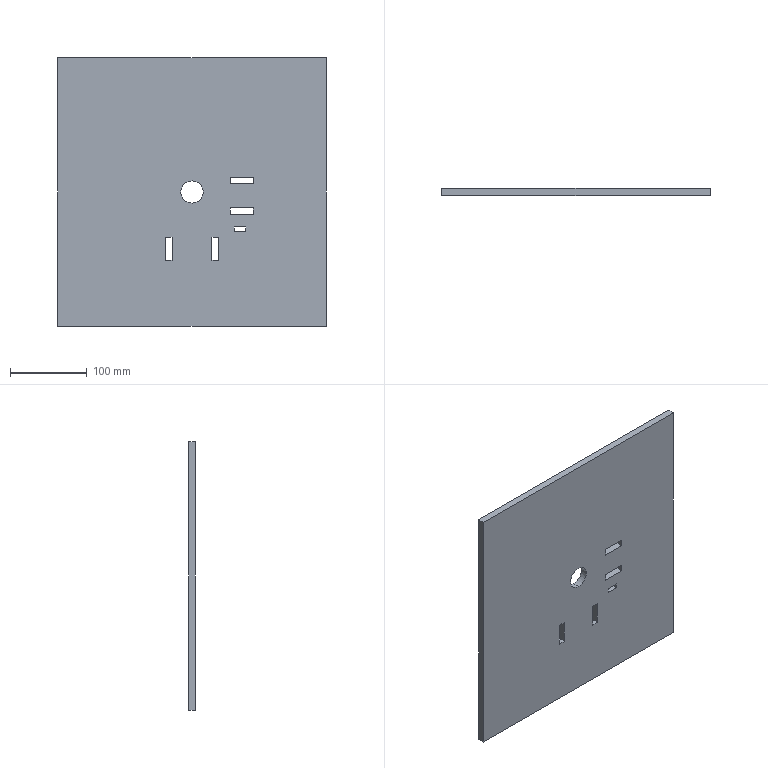Part | SolidWorks | features FlatPattern 1, ICE 1, SMBaseFlange 1, SheetMetal 1 | 1 solid | 28 faces | box 350 x 9 x 350 mm | volume 1086025 mm3 | plane 26 | cylinder 2 | commonest cylinder face diameters 29 x2
STEP:
#1=CARTESIAN_POINT('',(0.,9.,-14.5));
#2=VERTEX_POINT('',#1);
#3=CARTESIAN_POINT('',(0.,9.,14.5));
#4=VERTEX_POINT('',#3);
#5=CARTESIAN_POINT('',(0.,9.,0.));
#6=DIRECTION('',(0.,1.,0.));
#7=DIRECTION('',(0.,0.,1.));
#8=AXIS2_PLACEMENT_3D('',#5,#6,#7);
#9=CIRCLE('',#8,14.5);
#10=EDGE_CURVE('',#2,#4,#9,.T.);
#11=ORIENTED_EDGE('',*,*,#10,.T.);
#12=CARTESIAN_POINT('',(0.,0.,14.5));
#13=VERTEX_POINT('',#12);
#14=CARTESIAN_POINT('',(0.,9.,14.5));
#15=DIRECTION('',(0.,-1.,0.));
#16=VECTOR('',#15,1000.);
#17=LINE('',#14,#16);
#18=EDGE_CURVE('',#4,#13,#17,.T.);
#19=ORIENTED_EDGE('',*,*,#18,.T.);
#20=CARTESIAN_POINT('',(0.,0.,-14.5));
#21=VERTEX_POINT('',#20);
#22=CARTESIAN_POINT('',(0.,0.,0.));
#23=DIRECTION('',(0.,1.,0.));
#24=DIRECTION('',(0.,0.,1.));
#25=AXIS2_PLACEMENT_3D('',#22,#23,#24);
#26=CIRCLE('',#25,14.5);
#27=EDGE_CURVE('',#21,#13,#26,.T.);
#28=ORIENTED_EDGE('',*,*,#27,.F.);
#29=CARTESIAN_POINT('',(0.,9.,-14.5));
#30=DIRECTION('',(0.,-1.,0.));
#31=VECTOR('',#30,1000.);
#32=LINE('',#29,#31);
#33=EDGE_CURVE('',#2,#21,#32,.T.);
#34=ORIENTED_EDGE('',*,*,#33,.F.);
#35=EDGE_LOOP('',(#11,#19,#28,#34));
#36=FACE_OUTER_BOUND('',#35,.T.);
#37=CARTESIAN_POINT('',(0.,9.,0.));
#38=DIRECTION('',(0.,-1.,0.));
#39=DIRECTION('',(0.,0.,-1.));
#40=AXIS2_PLACEMENT_3D('',#37,#38,#39);
#41=CYLINDRICAL_SURFACE('',#40,14.5);
#42=ADVANCED_FACE('',(#36),#41,.F.);
#43=CARTESIAN_POINT('',(26.,9.,-59.));
#44=VERTEX_POINT('',#43);
#45=CARTESIAN_POINT('',(26.,9.,-89.));
#46=VERTEX_POINT('',#45);
#47=CARTESIAN_POINT('',(26.,9.,-59.));
#48=DIRECTION('',(0.,0.,-1.));
#49=VECTOR('',#48,1000.);
#50=LINE('',#47,#49);
#51=EDGE_CURVE('',#44,#46,#50,.T.);
#52=ORIENTED_EDGE('',*,*,#51,.T.);
#53=CARTESIAN_POINT('',(35.,9.,-89.));
#54=VERTEX_POINT('',#53);
#55=CARTESIAN_POINT('',(35.,9.,-89.));
#56=DIRECTION('',(1.,0.,0.));
#57=VECTOR('',#56,1000.);
#58=LINE('',#55,#57);
#59=EDGE_CURVE('',#46,#54,#58,.T.);
#60=ORIENTED_EDGE('',*,*,#59,.T.);
#61=CARTESIAN_POINT('',(35.,9.,-59.));
#62=VERTEX_POINT('',#61);
#63=CARTESIAN_POINT('',(35.,9.,-59.));
#64=DIRECTION('',(0.,0.,1.));
#65=VECTOR('',#64,1000.);
#66=LINE('',#63,#65);
#67=EDGE_CURVE('',#54,#62,#66,.T.);
#68=ORIENTED_EDGE('',*,*,#67,.T.);
#69=CARTESIAN_POINT('',(35.,9.,-59.));
#70=DIRECTION('',(-1.,0.,0.));
#71=VECTOR('',#70,1000.);
#72=LINE('',#69,#71);
#73=EDGE_CURVE('',#62,#44,#72,.T.);
#74=ORIENTED_EDGE('',*,*,#73,.T.);
#75=EDGE_LOOP('',(#52,#60,#68,#74));
#76=FACE_BOUND('',#75,.T.);
#77=CARTESIAN_POINT('',(80.,9.,10.5));
#78=VERTEX_POINT('',#77);
#79=CARTESIAN_POINT('',(80.,9.,19.5));
#80=VERTEX_POINT('',#79);
#81=CARTESIAN_POINT('',(80.,9.,19.5));
#82=DIRECTION('',(0.,0.,1.));
#83=VECTOR('',#82,1000.);
#84=LINE('',#81,#83);
#85=EDGE_CURVE('',#78,#80,#84,.T.);
#86=ORIENTED_EDGE('',*,*,#85,.T.);
#87=CARTESIAN_POINT('',(50.,9.,19.5));
#88=VERTEX_POINT('',#87);
#89=CARTESIAN_POINT('',(50.,9.,19.5));
#90=DIRECTION('',(-1.,0.,0.));
#91=VECTOR('',#90,1000.);
#92=LINE('',#89,#91);
#93=EDGE_CURVE('',#80,#88,#92,.T.);
#94=ORIENTED_EDGE('',*,*,#93,.T.);
#95=CARTESIAN_POINT('',(50.,9.,10.5));
#96=VERTEX_POINT('',#95);
#97=CARTESIAN_POINT('',(50.,9.,19.5));
#98=DIRECTION('',(0.,0.,-1.));
#99=VECTOR('',#98,1000.);
#100=LINE('',#97,#99);
#101=EDGE_CURVE('',#88,#96,#100,.T.);
#102=ORIENTED_EDGE('',*,*,#101,.T.);
#103=CARTESIAN_POINT('',(50.,9.,10.5));
#104=DIRECTION('',(1.,0.,0.));
#105=VECTOR('',#104,1000.);
#106=LINE('',#103,#105);
#107=EDGE_CURVE('',#96,#78,#106,.T.);
#108=ORIENTED_EDGE('',*,*,#107,.T.);
#109=EDGE_LOOP('',(#86,#94,#102,#108));
#110=FACE_BOUND('',#109,.T.);
#111=CARTESIAN_POINT('',(-35.,9.,-59.));
#112=VERTEX_POINT('',#111);
#113=CARTESIAN_POINT('',(-35.,9.,-89.));
#114=VERTEX_POINT('',#113);
#115=CARTESIAN_POINT('',(-35.,9.,-59.));
#116=DIRECTION('',(0.,0.,-1.));
#117=VECTOR('',#116,1000.);
#118=LINE('',#115,#117);
#119=EDGE_CURVE('',#112,#114,#118,.T.);
#120=ORIENTED_EDGE('',*,*,#119,.T.);
#121=CARTESIAN_POINT('',(-26.,9.,-89.));
#122=VERTEX_POINT('',#121);
#123=CARTESIAN_POINT('',(-35.,9.,-89.));
#124=DIRECTION('',(1.,0.,0.));
#125=VECTOR('',#124,1000.);
#126=LINE('',#123,#125);
#127=EDGE_CURVE('',#114,#122,#126,.T.);
#128=ORIENTED_EDGE('',*,*,#127,.T.);
#129=CARTESIAN_POINT('',(-26.,9.,-59.));
#130=VERTEX_POINT('',#129);
#131=CARTESIAN_POINT('',(-26.,9.,-59.));
#132=DIRECTION('',(0.,0.,1.));
#133=VECTOR('',#132,1000.);
#134=LINE('',#131,#133);
#135=EDGE_CURVE('',#122,#130,#134,.T.);
#136=ORIENTED_EDGE('',*,*,#135,.T.);
#137=CARTESIAN_POINT('',(-35.,9.,-59.));
#138=DIRECTION('',(-1.,0.,0.));
#139=VECTOR('',#138,1000.);
#140=LINE('',#137,#139);
#141=EDGE_CURVE('',#130,#112,#140,.T.);
#142=ORIENTED_EDGE('',*,*,#141,.T.);
#143=EDGE_LOOP('',(#120,#128,#136,#142));
#144=FACE_BOUND('',#143,.T.);
#145=CARTESIAN_POINT('',(55.,9.,-45.5));
#146=VERTEX_POINT('',#145);
#147=CARTESIAN_POINT('',(55.,9.,-51.5));
#148=VERTEX_POINT('',#147);
#149=CARTESIAN_POINT('',(55.,9.,-45.5));
#150=DIRECTION('',(0.,0.,-1.));
#151=VECTOR('',#150,1000.);
#152=LINE('',#149,#151);
#153=EDGE_CURVE('',#146,#148,#152,.T.);
#154=ORIENTED_EDGE('',*,*,#153,.T.);
#155=CARTESIAN_POINT('',(70.,9.,-51.5));
#156=VERTEX_POINT('',#155);
#157=CARTESIAN_POINT('',(70.,9.,-51.5));
#158=DIRECTION('',(1.,0.,0.));
#159=VECTOR('',#158,1000.);
#160=LINE('',#157,#159);
#161=EDGE_CURVE('',#148,#156,#160,.T.);
#162=ORIENTED_EDGE('',*,*,#161,.T.);
#163=CARTESIAN_POINT('',(70.,9.,-45.5));
#164=VERTEX_POINT('',#163);
#165=CARTESIAN_POINT('',(70.,9.,-45.5));
#166=DIRECTION('',(0.,0.,1.));
#167=VECTOR('',#166,1000.);
#168=LINE('',#165,#167);
#169=EDGE_CURVE('',#156,#164,#168,.T.);
#170=ORIENTED_EDGE('',*,*,#169,.T.);
#171=CARTESIAN_POINT('',(70.,9.,-45.5));
#172=DIRECTION('',(-1.,0.,0.));
#173=VECTOR('',#172,1000.);
#174=LINE('',#171,#173);
#175=EDGE_CURVE('',#164,#146,#174,.T.);
#176=ORIENTED_EDGE('',*,*,#175,.T.);
#177=EDGE_LOOP('',(#154,#162,#170,#176));
#178=FACE_BOUND('',#177,.T.);
#179=CARTESIAN_POINT('',(80.,9.,-29.5));
#180=VERTEX_POINT('',#179);
#181=CARTESIAN_POINT('',(80.,9.,-20.5));
#182=VERTEX_POINT('',#181);
#183=CARTESIAN_POINT('',(80.,9.,-20.5));
#184=DIRECTION('',(0.,0.,1.));
#185=VECTOR('',#184,1000.);
#186=LINE('',#183,#185);
#187=EDGE_CURVE('',#180,#182,#186,.T.);
#188=ORIENTED_EDGE('',*,*,#187,.T.);
#189=CARTESIAN_POINT('',(50.,9.,-20.5));
#190=VERTEX_POINT('',#189);
#191=CARTESIAN_POINT('',(50.,9.,-20.5));
#192=DIRECTION('',(-1.,0.,0.));
#193=VECTOR('',#192,1000.);
#194=LINE('',#191,#193);
#195=EDGE_CURVE('',#182,#190,#194,.T.);
#196=ORIENTED_EDGE('',*,*,#195,.T.);
#197=CARTESIAN_POINT('',(50.,9.,-29.5));
#198=VERTEX_POINT('',#197);
#199=CARTESIAN_POINT('',(50.,9.,-20.5));
#200=DIRECTION('',(0.,0.,-1.));
#201=VECTOR('',#200,1000.);
#202=LINE('',#199,#201);
#203=EDGE_CURVE('',#190,#198,#202,.T.);
#204=ORIENTED_EDGE('',*,*,#203,.T.);
#205=CARTESIAN_POINT('',(50.,9.,-29.5));
#206=DIRECTION('',(1.,0.,0.));
#207=VECTOR('',#206,1000.);
#208=LINE('',#205,#207);
#209=EDGE_CURVE('',#198,#180,#208,.T.);
#210=ORIENTED_EDGE('',*,*,#209,.T.);
#211=EDGE_LOOP('',(#188,#196,#204,#210));
#212=FACE_BOUND('',#211,.T.);
#213=CARTESIAN_POINT('',(175.,9.,175.));
#214=VERTEX_POINT('',#213);
#215=CARTESIAN_POINT('',(175.,9.,-175.));
#216=VERTEX_POINT('',#215);
#217=CARTESIAN_POINT('',(175.,9.,-175.));
#218=DIRECTION('',(0.,0.,-1.));
#219=VECTOR('',#218,1000.);
#220=LINE('',#217,#219);
#221=EDGE_CURVE('',#214,#216,#220,.T.);
#222=ORIENTED_EDGE('',*,*,#221,.T.);
#223=CARTESIAN_POINT('',(-175.,9.,-175.));
#224=VERTEX_POINT('',#223);
#225=CARTESIAN_POINT('',(-175.,9.,-175.));
#226=DIRECTION('',(-1.,0.,0.));
#227=VECTOR('',#226,1000.);
#228=LINE('',#225,#227);
#229=EDGE_CURVE('',#216,#224,#228,.T.);
#230=ORIENTED_EDGE('',*,*,#229,.T.);
#231=CARTESIAN_POINT('',(-175.,9.,175.));
#232=VERTEX_POINT('',#231);
#233=CARTESIAN_POINT('',(-175.,9.,-175.));
#234=DIRECTION('',(0.,0.,1.));
#235=VECTOR('',#234,1000.);
#236=LINE('',#233,#235);
#237=EDGE_CURVE('',#224,#232,#236,.T.);
#238=ORIENTED_EDGE('',*,*,#237,.T.);
#239=CARTESIAN_POINT('',(-175.,9.,175.));
#240=DIRECTION('',(1.,0.,0.));
#241=VECTOR('',#240,1000.);
#242=LINE('',#239,#241);
#243=EDGE_CURVE('',#232,#214,#242,.T.);
#244=ORIENTED_EDGE('',*,*,#243,.T.);
#245=EDGE_LOOP('',(#222,#230,#238,#244));
#246=FACE_OUTER_BOUND('',#245,.T.);
#247=ORIENTED_EDGE('',*,*,#10,.F.);
#248=CARTESIAN_POINT('',(0.,9.,0.));
#249=DIRECTION('',(0.,1.,0.));
#250=DIRECTION('',(0.,0.,1.));
#251=AXIS2_PLACEMENT_3D('',#248,#249,#250);
#252=CIRCLE('',#251,14.5);
#253=EDGE_CURVE('',#4,#2,#252,.T.);
#254=ORIENTED_EDGE('',*,*,#253,.F.);
#255=EDGE_LOOP('',(#247,#254));
#256=FACE_BOUND('',#255,.T.);
#257=CARTESIAN_POINT('',(0.,9.,0.));
#258=DIRECTION('',(0.,1.,0.));
#259=DIRECTION('',(0.,0.,1.));
#260=AXIS2_PLACEMENT_3D('',#257,#258,#259);
#261=PLANE('',#260);
#262=ADVANCED_FACE('',(#76,#110,#144,#178,#212,#246,#256),#261,.T.);
#263=CARTESIAN_POINT('',(26.,0.,-89.));
#264=VERTEX_POINT('',#263);
#265=CARTESIAN_POINT('',(35.,0.,-89.));
#266=VERTEX_POINT('',#265);
#267=CARTESIAN_POINT('',(35.,0.,-89.));
#268=DIRECTION('',(1.,0.,0.));
#269=VECTOR('',#268,1000.);
#270=LINE('',#267,#269);
#271=EDGE_CURVE('',#264,#266,#270,.T.);
#272=ORIENTED_EDGE('',*,*,#271,.F.);
#273=CARTESIAN_POINT('',(26.,0.,-59.));
#274=VERTEX_POINT('',#273);
#275=CARTESIAN_POINT('',(26.,0.,-59.));
#276=DIRECTION('',(0.,0.,-1.));
#277=VECTOR('',#276,1000.);
#278=LINE('',#275,#277);
#279=EDGE_CURVE('',#274,#264,#278,.T.);
#280=ORIENTED_EDGE('',*,*,#279,.F.);
#281=CARTESIAN_POINT('',(35.,0.,-59.));
#282=VERTEX_POINT('',#281);
#283=CARTESIAN_POINT('',(35.,0.,-59.));
#284=DIRECTION('',(-1.,0.,0.));
#285=VECTOR('',#284,1000.);
#286=LINE('',#283,#285);
#287=EDGE_CURVE('',#282,#274,#286,.T.);
#288=ORIENTED_EDGE('',*,*,#287,.F.);
#289=CARTESIAN_POINT('',(35.,0.,-59.));
#290=DIRECTION('',(0.,0.,1.));
#291=VECTOR('',#290,1000.);
#292=LINE('',#289,#291);
#293=EDGE_CURVE('',#266,#282,#292,.T.);
#294=ORIENTED_EDGE('',*,*,#293,.F.);
#295=EDGE_LOOP('',(#272,#280,#288,#294));
#296=FACE_BOUND('',#295,.T.);
#297=CARTESIAN_POINT('',(80.,0.,19.5));
#298=VERTEX_POINT('',#297);
#299=CARTESIAN_POINT('',(50.,0.,19.5));
#300=VERTEX_POINT('',#299);
#301=CARTESIAN_POINT('',(50.,0.,19.5));
#302=DIRECTION('',(-1.,0.,0.));
#303=VECTOR('',#302,1000.);
#304=LINE('',#301,#303);
#305=EDGE_CURVE('',#298,#300,#304,.T.);
#306=ORIENTED_EDGE('',*,*,#305,.F.);
#307=CARTESIAN_POINT('',(80.,0.,10.5));
#308=VERTEX_POINT('',#307);
#309=CARTESIAN_POINT('',(80.,0.,19.5));
#310=DIRECTION('',(0.,0.,1.));
#311=VECTOR('',#310,1000.);
#312=LINE('',#309,#311);
#313=EDGE_CURVE('',#308,#298,#312,.T.);
#314=ORIENTED_EDGE('',*,*,#313,.F.);
#315=CARTESIAN_POINT('',(50.,0.,10.5));
#316=VERTEX_POINT('',#315);
#317=CARTESIAN_POINT('',(50.,0.,10.5));
#318=DIRECTION('',(1.,0.,0.));
#319=VECTOR('',#318,1000.);
#320=LINE('',#317,#319);
#321=EDGE_CURVE('',#316,#308,#320,.T.);
#322=ORIENTED_EDGE('',*,*,#321,.F.);
#323=CARTESIAN_POINT('',(50.,0.,19.5));
#324=DIRECTION('',(0.,0.,-1.));
#325=VECTOR('',#324,1000.);
#326=LINE('',#323,#325);
#327=EDGE_CURVE('',#300,#316,#326,.T.);
#328=ORIENTED_EDGE('',*,*,#327,.F.);
#329=EDGE_LOOP('',(#306,#314,#322,#328));
#330=FACE_BOUND('',#329,.T.);
#331=CARTESIAN_POINT('',(-35.,0.,-89.));
#332=VERTEX_POINT('',#331);
#333=CARTESIAN_POINT('',(-26.,0.,-89.));
#334=VERTEX_POINT('',#333);
#335=CARTESIAN_POINT('',(-35.,0.,-89.));
#336=DIRECTION('',(1.,0.,0.));
#337=VECTOR('',#336,1000.);
#338=LINE('',#335,#337);
#339=EDGE_CURVE('',#332,#334,#338,.T.);
#340=ORIENTED_EDGE('',*,*,#339,.F.);
#341=CARTESIAN_POINT('',(-35.,0.,-59.));
#342=VERTEX_POINT('',#341);
#343=CARTESIAN_POINT('',(-35.,0.,-59.));
#344=DIRECTION('',(0.,0.,-1.));
#345=VECTOR('',#344,1000.);
#346=LINE('',#343,#345);
#347=EDGE_CURVE('',#342,#332,#346,.T.);
#348=ORIENTED_EDGE('',*,*,#347,.F.);
#349=CARTESIAN_POINT('',(-26.,0.,-59.));
#350=VERTEX_POINT('',#349);
#351=CARTESIAN_POINT('',(-35.,0.,-59.));
#352=DIRECTION('',(-1.,0.,0.));
#353=VECTOR('',#352,1000.);
#354=LINE('',#351,#353);
#355=EDGE_CURVE('',#350,#342,#354,.T.);
#356=ORIENTED_EDGE('',*,*,#355,.F.);
#357=CARTESIAN_POINT('',(-26.,0.,-59.));
#358=DIRECTION('',(0.,0.,1.));
#359=VECTOR('',#358,1000.);
#360=LINE('',#357,#359);
#361=EDGE_CURVE('',#334,#350,#360,.T.);
#362=ORIENTED_EDGE('',*,*,#361,.F.);
#363=EDGE_LOOP('',(#340,#348,#356,#362));
#364=FACE_BOUND('',#363,.T.);
#365=CARTESIAN_POINT('',(55.,0.,-51.5));
#366=VERTEX_POINT('',#365);
#367=CARTESIAN_POINT('',(70.,0.,-51.5));
#368=VERTEX_POINT('',#367);
#369=CARTESIAN_POINT('',(70.,0.,-51.5));
#370=DIRECTION('',(1.,0.,0.));
#371=VECTOR('',#370,1000.);
#372=LINE('',#369,#371);
#373=EDGE_CURVE('',#366,#368,#372,.T.);
#374=ORIENTED_EDGE('',*,*,#373,.F.);
#375=CARTESIAN_POINT('',(55.,0.,-45.5));
#376=VERTEX_POINT('',#375);
#377=CARTESIAN_POINT('',(55.,0.,-45.5));
#378=DIRECTION('',(0.,0.,-1.));
#379=VECTOR('',#378,1000.);
#380=LINE('',#377,#379);
#381=EDGE_CURVE('',#376,#366,#380,.T.);
#382=ORIENTED_EDGE('',*,*,#381,.F.);
#383=CARTESIAN_POINT('',(70.,0.,-45.5));
#384=VERTEX_POINT('',#383);
#385=CARTESIAN_POINT('',(70.,0.,-45.5));
#386=DIRECTION('',(-1.,0.,0.));
#387=VECTOR('',#386,1000.);
#388=LINE('',#385,#387);
#389=EDGE_CURVE('',#384,#376,#388,.T.);
#390=ORIENTED_EDGE('',*,*,#389,.F.);
#391=CARTESIAN_POINT('',(70.,0.,-45.5));
#392=DIRECTION('',(0.,0.,1.));
#393=VECTOR('',#392,1000.);
#394=LINE('',#391,#393);
#395=EDGE_CURVE('',#368,#384,#394,.T.);
#396=ORIENTED_EDGE('',*,*,#395,.F.);
#397=EDGE_LOOP('',(#374,#382,#390,#396));
#398=FACE_BOUND('',#397,.T.);
#399=CARTESIAN_POINT('',(80.,0.,-20.5));
#400=VERTEX_POINT('',#399);
#401=CARTESIAN_POINT('',(50.,0.,-20.5));
#402=VERTEX_POINT('',#401);
#403=CARTESIAN_POINT('',(50.,0.,-20.5));
#404=DIRECTION('',(-1.,0.,0.));
#405=VECTOR('',#404,1000.);
#406=LINE('',#403,#405);
#407=EDGE_CURVE('',#400,#402,#406,.T.);
#408=ORIENTED_EDGE('',*,*,#407,.F.);
#409=CARTESIAN_POINT('',(80.,0.,-29.5));
#410=VERTEX_POINT('',#409);
#411=CARTESIAN_POINT('',(80.,0.,-20.5));
#412=DIRECTION('',(0.,0.,1.));
#413=VECTOR('',#412,1000.);
#414=LINE('',#411,#413);
#415=EDGE_CURVE('',#410,#400,#414,.T.);
#416=ORIENTED_EDGE('',*,*,#415,.F.);
#417=CARTESIAN_POINT('',(50.,0.,-29.5));
#418=VERTEX_POINT('',#417);
#419=CARTESIAN_POINT('',(50.,0.,-29.5));
#420=DIRECTION('',(1.,0.,0.));
#421=VECTOR('',#420,1000.);
#422=LINE('',#419,#421);
#423=EDGE_CURVE('',#418,#410,#422,.T.);
#424=ORIENTED_EDGE('',*,*,#423,.F.);
#425=CARTESIAN_POINT('',(50.,0.,-20.5));
#426=DIRECTION('',(0.,0.,-1.));
#427=VECTOR('',#426,1000.);
#428=LINE('',#425,#427);
#429=EDGE_CURVE('',#402,#418,#428,.T.);
#430=ORIENTED_EDGE('',*,*,#429,.F.);
#431=EDGE_LOOP('',(#408,#416,#424,#430));
#432=FACE_BOUND('',#431,.T.);
#433=CARTESIAN_POINT('',(175.,0.,175.));
#434=VERTEX_POINT('',#433);
#435=CARTESIAN_POINT('',(175.,0.,-175.));
#436=VERTEX_POINT('',#435);
#437=CARTESIAN_POINT('',(175.,0.,-175.));
#438=DIRECTION('',(0.,0.,-1.));
#439=VECTOR('',#438,1000.);
#440=LINE('',#437,#439);
#441=EDGE_CURVE('',#434,#436,#440,.T.);
#442=ORIENTED_EDGE('',*,*,#441,.F.);
#443=CARTESIAN_POINT('',(-175.,0.,175.));
#444=VERTEX_POINT('',#443);
#445=CARTESIAN_POINT('',(-175.,0.,175.));
#446=DIRECTION('',(1.,0.,0.));
#447=VECTOR('',#446,1000.);
#448=LINE('',#445,#447);
#449=EDGE_CURVE('',#444,#434,#448,.T.);
#450=ORIENTED_EDGE('',*,*,#449,.F.);
#451=CARTESIAN_POINT('',(-175.,0.,-175.));
#452=VERTEX_POINT('',#451);
#453=CARTESIAN_POINT('',(-175.,0.,-175.));
#454=DIRECTION('',(0.,0.,1.));
#455=VECTOR('',#454,1000.);
#456=LINE('',#453,#455);
#457=EDGE_CURVE('',#452,#444,#456,.T.);
#458=ORIENTED_EDGE('',*,*,#457,.F.);
#459=CARTESIAN_POINT('',(-175.,0.,-175.));
#460=DIRECTION('',(-1.,0.,0.));
#461=VECTOR('',#460,1000.);
#462=LINE('',#459,#461);
#463=EDGE_CURVE('',#436,#452,#462,.T.);
#464=ORIENTED_EDGE('',*,*,#463,.F.);
#465=EDGE_LOOP('',(#442,#450,#458,#464));
#466=FACE_OUTER_BOUND('',#465,.T.);
#467=ORIENTED_EDGE('',*,*,#27,.T.);
#468=CARTESIAN_POINT('',(0.,0.,0.));
#469=DIRECTION('',(0.,1.,0.));
#470=DIRECTION('',(0.,0.,1.));
#471=AXIS2_PLACEMENT_3D('',#468,#469,#470);
#472=CIRCLE('',#471,14.5);
#473=EDGE_CURVE('',#13,#21,#472,.T.);
#474=ORIENTED_EDGE('',*,*,#473,.T.);
#475=EDGE_LOOP('',(#467,#474));
#476=FACE_BOUND('',#475,.T.);
#477=CARTESIAN_POINT('',(0.,0.,0.));
#478=DIRECTION('',(0.,1.,0.));
#479=DIRECTION('',(0.,0.,1.));
#480=AXIS2_PLACEMENT_3D('',#477,#478,#479);
#481=PLANE('',#480);
#482=ADVANCED_FACE('',(#296,#330,#364,#398,#432,#466,#476),#481,.F.);
#483=ORIENTED_EDGE('',*,*,#441,.T.);
#484=CARTESIAN_POINT('',(175.,9.,-175.));
#485=DIRECTION('',(0.,-1.,0.));
#486=VECTOR('',#485,1000.);
#487=LINE('',#484,#486);
#488=EDGE_CURVE('',#216,#436,#487,.T.);
#489=ORIENTED_EDGE('',*,*,#488,.F.);
#490=ORIENTED_EDGE('',*,*,#221,.F.);
#491=CARTESIAN_POINT('',(175.,9.,175.));
#492=DIRECTION('',(0.,-1.,0.));
#493=VECTOR('',#492,1000.);
#494=LINE('',#491,#493);
#495=EDGE_CURVE('',#214,#434,#494,.T.);
#496=ORIENTED_EDGE('',*,*,#495,.T.);
#497=EDGE_LOOP('',(#483,#489,#490,#496));
#498=FACE_OUTER_BOUND('',#497,.T.);
#499=CARTESIAN_POINT('',(175.,9.,-175.));
#500=DIRECTION('',(-1.,0.,0.));
#501=DIRECTION('',(0.,0.,1.));
#502=AXIS2_PLACEMENT_3D('',#499,#500,#501);
#503=PLANE('',#502);
#504=ADVANCED_FACE('',(#498),#503,.F.);
#505=ORIENTED_EDGE('',*,*,#463,.T.);
#506=CARTESIAN_POINT('',(-175.,9.,-175.));
#507=DIRECTION('',(0.,-1.,0.));
#508=VECTOR('',#507,1000.);
#509=LINE('',#506,#508);
#510=EDGE_CURVE('',#224,#452,#509,.T.);
#511=ORIENTED_EDGE('',*,*,#510,.F.);
#512=ORIENTED_EDGE('',*,*,#229,.F.);
#513=ORIENTED_EDGE('',*,*,#488,.T.);
#514=EDGE_LOOP('',(#505,#511,#512,#513));
#515=FACE_OUTER_BOUND('',#514,.T.);
#516=CARTESIAN_POINT('',(-175.,9.,-175.));
#517=DIRECTION('',(0.,0.,1.));
#518=DIRECTION('',(1.,0.,0.));
#519=AXIS2_PLACEMENT_3D('',#516,#517,#518);
#520=PLANE('',#519);
#521=ADVANCED_FACE('',(#515),#520,.F.);
#522=ORIENTED_EDGE('',*,*,#457,.T.);
#523=CARTESIAN_POINT('',(-175.,9.,175.));
#524=DIRECTION('',(0.,-1.,0.));
#525=VECTOR('',#524,1000.);
#526=LINE('',#523,#525);
#527=EDGE_CURVE('',#232,#444,#526,.T.);
#528=ORIENTED_EDGE('',*,*,#527,.F.);
#529=ORIENTED_EDGE('',*,*,#237,.F.);
#530=ORIENTED_EDGE('',*,*,#510,.T.);
#531=EDGE_LOOP('',(#522,#528,#529,#530));
#532=FACE_OUTER_BOUND('',#531,.T.);
#533=CARTESIAN_POINT('',(-175.,9.,-175.));
#534=DIRECTION('',(1.,0.,0.));
#535=DIRECTION('',(0.,0.,-1.));
#536=AXIS2_PLACEMENT_3D('',#533,#534,#535);
#537=PLANE('',#536);
#538=ADVANCED_FACE('',(#532),#537,.F.);
#539=ORIENTED_EDGE('',*,*,#449,.T.);
#540=ORIENTED_EDGE('',*,*,#495,.F.);
#541=ORIENTED_EDGE('',*,*,#243,.F.);
#542=ORIENTED_EDGE('',*,*,#527,.T.);
#543=EDGE_LOOP('',(#539,#540,#541,#542));
#544=FACE_OUTER_BOUND('',#543,.T.);
#545=CARTESIAN_POINT('',(-175.,9.,175.));
#546=DIRECTION('',(0.,0.,-1.));
#547=DIRECTION('',(-1.,0.,0.));
#548=AXIS2_PLACEMENT_3D('',#545,#546,#547);
#549=PLANE('',#548);
#550=ADVANCED_FACE('',(#544),#549,.F.);
#551=ORIENTED_EDGE('',*,*,#18,.F.);
#552=ORIENTED_EDGE('',*,*,#253,.T.);
#553=ORIENTED_EDGE('',*,*,#33,.T.);
#554=ORIENTED_EDGE('',*,*,#473,.F.);
#555=EDGE_LOOP('',(#551,#552,#553,#554));
#556=FACE_OUTER_BOUND('',#555,.T.);
#557=CARTESIAN_POINT('',(0.,9.,0.));
#558=DIRECTION('',(0.,-1.,0.));
#559=DIRECTION('',(0.,0.,-1.));
#560=AXIS2_PLACEMENT_3D('',#557,#558,#559);
#561=CYLINDRICAL_SURFACE('',#560,14.5);
#562=ADVANCED_FACE('',(#556),#561,.F.);
#563=ORIENTED_EDGE('',*,*,#415,.T.);
#564=CARTESIAN_POINT('',(80.,9.,-20.5));
#565=DIRECTION('',(0.,-1.,0.));
#566=VECTOR('',#565,1000.);
#567=LINE('',#564,#566);
#568=EDGE_CURVE('',#182,#400,#567,.T.);
#569=ORIENTED_EDGE('',*,*,#568,.F.);
#570=ORIENTED_EDGE('',*,*,#187,.F.);
#571=CARTESIAN_POINT('',(80.,9.,-29.5));
#572=DIRECTION('',(0.,-1.,0.));
#573=VECTOR('',#572,1000.);
#574=LINE('',#571,#573);
#575=EDGE_CURVE('',#180,#410,#574,.T.);
#576=ORIENTED_EDGE('',*,*,#575,.T.);
#577=EDGE_LOOP('',(#563,#569,#570,#576));
#578=FACE_OUTER_BOUND('',#577,.T.);
#579=CARTESIAN_POINT('',(80.,9.,-20.5));
#580=DIRECTION('',(1.,0.,0.));
#581=DIRECTION('',(0.,0.,-1.));
#582=AXIS2_PLACEMENT_3D('',#579,#580,#581);
#583=PLANE('',#582);
#584=ADVANCED_FACE('',(#578),#583,.F.);
#585=ORIENTED_EDGE('',*,*,#423,.T.);
#586=ORIENTED_EDGE('',*,*,#575,.F.);
#587=ORIENTED_EDGE('',*,*,#209,.F.);
#588=CARTESIAN_POINT('',(50.,9.,-29.5));
#589=DIRECTION('',(0.,-1.,0.));
#590=VECTOR('',#589,1000.);
#591=LINE('',#588,#590);
#592=EDGE_CURVE('',#198,#418,#591,.T.);
#593=ORIENTED_EDGE('',*,*,#592,.T.);
#594=EDGE_LOOP('',(#585,#586,#587,#593));
#595=FACE_OUTER_BOUND('',#594,.T.);
#596=CARTESIAN_POINT('',(50.,9.,-29.5));
#597=DIRECTION('',(0.,0.,-1.));
#598=DIRECTION('',(-1.,0.,0.));
#599=AXIS2_PLACEMENT_3D('',#596,#597,#598);
#600=PLANE('',#599);
#601=ADVANCED_FACE('',(#595),#600,.F.);
#602=ORIENTED_EDGE('',*,*,#429,.T.);
#603=ORIENTED_EDGE('',*,*,#592,.F.);
#604=ORIENTED_EDGE('',*,*,#203,.F.);
#605=CARTESIAN_POINT('',(50.,9.,-20.5));
#606=DIRECTION('',(0.,-1.,0.));
#607=VECTOR('',#606,1000.);
#608=LINE('',#605,#607);
#609=EDGE_CURVE('',#190,#402,#608,.T.);
#610=ORIENTED_EDGE('',*,*,#609,.T.);
#611=EDGE_LOOP('',(#602,#603,#604,#610));
#612=FACE_OUTER_BOUND('',#611,.T.);
#613=CARTESIAN_POINT('',(50.,9.,-20.5));
#614=DIRECTION('',(-1.,0.,0.));
#615=DIRECTION('',(0.,0.,1.));
#616=AXIS2_PLACEMENT_3D('',#613,#614,#615);
#617=PLANE('',#616);
#618=ADVANCED_FACE('',(#612),#617,.F.);
#619=ORIENTED_EDGE('',*,*,#407,.T.);
#620=ORIENTED_EDGE('',*,*,#609,.F.);
#621=ORIENTED_EDGE('',*,*,#195,.F.);
#622=ORIENTED_EDGE('',*,*,#568,.T.);
#623=EDGE_LOOP('',(#619,#620,#621,#622));
#624=FACE_OUTER_BOUND('',#623,.T.);
#625=CARTESIAN_POINT('',(50.,9.,-20.5));
#626=DIRECTION('',(0.,0.,1.));
#627=DIRECTION('',(1.,0.,0.));
#628=AXIS2_PLACEMENT_3D('',#625,#626,#627);
#629=PLANE('',#628);
#630=ADVANCED_FACE('',(#624),#629,.F.);
#631=ORIENTED_EDGE('',*,*,#381,.T.);
#632=CARTESIAN_POINT('',(55.,9.,-51.5));
#633=DIRECTION('',(0.,-1.,0.));
#634=VECTOR('',#633,1000.);
#635=LINE('',#632,#634);
#636=EDGE_CURVE('',#148,#366,#635,.T.);
#637=ORIENTED_EDGE('',*,*,#636,.F.);
#638=ORIENTED_EDGE('',*,*,#153,.F.);
#639=CARTESIAN_POINT('',(55.,9.,-45.5));
#640=DIRECTION('',(0.,-1.,0.));
#641=VECTOR('',#640,1000.);
#642=LINE('',#639,#641);
#643=EDGE_CURVE('',#146,#376,#642,.T.);
#644=ORIENTED_EDGE('',*,*,#643,.T.);
#645=EDGE_LOOP('',(#631,#637,#638,#644));
#646=FACE_OUTER_BOUND('',#645,.T.);
#647=CARTESIAN_POINT('',(55.,9.,-45.5));
#648=DIRECTION('',(-1.,0.,0.));
#649=DIRECTION('',(0.,0.,1.));
#650=AXIS2_PLACEMENT_3D('',#647,#648,#649);
#651=PLANE('',#650);
#652=ADVANCED_FACE('',(#646),#651,.F.);
#653=ORIENTED_EDGE('',*,*,#389,.T.);
#654=ORIENTED_EDGE('',*,*,#643,.F.);
#655=ORIENTED_EDGE('',*,*,#175,.F.);
#656=CARTESIAN_POINT('',(70.,9.,-45.5));
#657=DIRECTION('',(0.,-1.,0.));
#658=VECTOR('',#657,1000.);
#659=LINE('',#656,#658);
#660=EDGE_CURVE('',#164,#384,#659,.T.);
#661=ORIENTED_EDGE('',*,*,#660,.T.);
#662=EDGE_LOOP('',(#653,#654,#655,#661));
#663=FACE_OUTER_BOUND('',#662,.T.);
#664=CARTESIAN_POINT('',(70.,9.,-45.5));
#665=DIRECTION('',(0.,0.,1.));
#666=DIRECTION('',(1.,0.,0.));
#667=AXIS2_PLACEMENT_3D('',#664,#665,#666);
#668=PLANE('',#667);
#669=ADVANCED_FACE('',(#663),#668,.F.);
#670=ORIENTED_EDGE('',*,*,#395,.T.);
#671=ORIENTED_EDGE('',*,*,#660,.F.);
#672=ORIENTED_EDGE('',*,*,#169,.F.);
#673=CARTESIAN_POINT('',(70.,9.,-51.5));
#674=DIRECTION('',(0.,-1.,0.));
#675=VECTOR('',#674,1000.);
#676=LINE('',#673,#675);
#677=EDGE_CURVE('',#156,#368,#676,.T.);
#678=ORIENTED_EDGE('',*,*,#677,.T.);
#679=EDGE_LOOP('',(#670,#671,#672,#678));
#680=FACE_OUTER_BOUND('',#679,.T.);
#681=CARTESIAN_POINT('',(70.,9.,-45.5));
#682=DIRECTION('',(1.,0.,0.));
#683=DIRECTION('',(0.,0.,-1.));
#684=AXIS2_PLACEMENT_3D('',#681,#682,#683);
#685=PLANE('',#684);
#686=ADVANCED_FACE('',(#680),#685,.F.);
#687=ORIENTED_EDGE('',*,*,#373,.T.);
#688=ORIENTED_EDGE('',*,*,#677,.F.);
#689=ORIENTED_EDGE('',*,*,#161,.F.);
#690=ORIENTED_EDGE('',*,*,#636,.T.);
#691=EDGE_LOOP('',(#687,#688,#689,#690));
#692=FACE_OUTER_BOUND('',#691,.T.);
#693=CARTESIAN_POINT('',(70.,9.,-51.5));
#694=DIRECTION('',(0.,0.,-1.));
#695=DIRECTION('',(-1.,0.,0.));
#696=AXIS2_PLACEMENT_3D('',#693,#694,#695);
#697=PLANE('',#696);
#698=ADVANCED_FACE('',(#692),#697,.F.);
#699=ORIENTED_EDGE('',*,*,#347,.T.);
#700=CARTESIAN_POINT('',(-35.,9.,-89.));
#701=DIRECTION('',(0.,-1.,0.));
#702=VECTOR('',#701,1000.);
#703=LINE('',#700,#702);
#704=EDGE_CURVE('',#114,#332,#703,.T.);
#705=ORIENTED_EDGE('',*,*,#704,.F.);
#706=ORIENTED_EDGE('',*,*,#119,.F.);
#707=CARTESIAN_POINT('',(-35.,9.,-59.));
#708=DIRECTION('',(0.,-1.,0.));
#709=VECTOR('',#708,1000.);
#710=LINE('',#707,#709);
#711=EDGE_CURVE('',#112,#342,#710,.T.);
#712=ORIENTED_EDGE('',*,*,#711,.T.);
#713=EDGE_LOOP('',(#699,#705,#706,#712));
#714=FACE_OUTER_BOUND('',#713,.T.);
#715=CARTESIAN_POINT('',(-35.,9.,-59.));
#716=DIRECTION('',(-1.,0.,0.));
#717=DIRECTION('',(0.,0.,1.));
#718=AXIS2_PLACEMENT_3D('',#715,#716,#717);
#719=PLANE('',#718);
#720=ADVANCED_FACE('',(#714),#719,.F.);
#721=ORIENTED_EDGE('',*,*,#355,.T.);
#722=ORIENTED_EDGE('',*,*,#711,.F.);
#723=ORIENTED_EDGE('',*,*,#141,.F.);
#724=CARTESIAN_POINT('',(-26.,9.,-59.));
#725=DIRECTION('',(0.,-1.,0.));
#726=VECTOR('',#725,1000.);
#727=LINE('',#724,#726);
#728=EDGE_CURVE('',#130,#350,#727,.T.);
#729=ORIENTED_EDGE('',*,*,#728,.T.);
#730=EDGE_LOOP('',(#721,#722,#723,#729));
#731=FACE_OUTER_BOUND('',#730,.T.);
#732=CARTESIAN_POINT('',(-35.,9.,-59.));
#733=DIRECTION('',(0.,0.,1.));
#734=DIRECTION('',(1.,0.,0.));
#735=AXIS2_PLACEMENT_3D('',#732,#733,#734);
#736=PLANE('',#735);
#737=ADVANCED_FACE('',(#731),#736,.F.);
#738=ORIENTED_EDGE('',*,*,#361,.T.);
#739=ORIENTED_EDGE('',*,*,#728,.F.);
#740=ORIENTED_EDGE('',*,*,#135,.F.);
#741=CARTESIAN_POINT('',(-26.,9.,-89.));
#742=DIRECTION('',(0.,-1.,0.));
#743=VECTOR('',#742,1000.);
#744=LINE('',#741,#743);
#745=EDGE_CURVE('',#122,#334,#744,.T.);
#746=ORIENTED_EDGE('',*,*,#745,.T.);
#747=EDGE_LOOP('',(#738,#739,#740,#746));
#748=FACE_OUTER_BOUND('',#747,.T.);
#749=CARTESIAN_POINT('',(-26.,9.,-59.));
#750=DIRECTION('',(1.,0.,0.));
#751=DIRECTION('',(0.,0.,-1.));
#752=AXIS2_PLACEMENT_3D('',#749,#750,#751);
#753=PLANE('',#752);
#754=ADVANCED_FACE('',(#748),#753,.F.);
#755=ORIENTED_EDGE('',*,*,#339,.T.);
#756=ORIENTED_EDGE('',*,*,#745,.F.);
#757=ORIENTED_EDGE('',*,*,#127,.F.);
#758=ORIENTED_EDGE('',*,*,#704,.T.);
#759=EDGE_LOOP('',(#755,#756,#757,#758));
#760=FACE_OUTER_BOUND('',#759,.T.);
#761=CARTESIAN_POINT('',(-35.,9.,-89.));
#762=DIRECTION('',(0.,0.,-1.));
#763=DIRECTION('',(-1.,0.,0.));
#764=AXIS2_PLACEMENT_3D('',#761,#762,#763);
#765=PLANE('',#764);
#766=ADVANCED_FACE('',(#760),#765,.F.);
#767=ORIENTED_EDGE('',*,*,#313,.T.);
#768=CARTESIAN_POINT('',(80.,9.,19.5));
#769=DIRECTION('',(0.,-1.,0.));
#770=VECTOR('',#769,1000.);
#771=LINE('',#768,#770);
#772=EDGE_CURVE('',#80,#298,#771,.T.);
#773=ORIENTED_EDGE('',*,*,#772,.F.);
#774=ORIENTED_EDGE('',*,*,#85,.F.);
#775=CARTESIAN_POINT('',(80.,9.,10.5));
#776=DIRECTION('',(0.,-1.,0.));
#777=VECTOR('',#776,1000.);
#778=LINE('',#775,#777);
#779=EDGE_CURVE('',#78,#308,#778,.T.);
#780=ORIENTED_EDGE('',*,*,#779,.T.);
#781=EDGE_LOOP('',(#767,#773,#774,#780));
#782=FACE_OUTER_BOUND('',#781,.T.);
#783=CARTESIAN_POINT('',(80.,9.,19.5));
#784=DIRECTION('',(1.,0.,0.));
#785=DIRECTION('',(0.,0.,-1.));
#786=AXIS2_PLACEMENT_3D('',#783,#784,#785);
#787=PLANE('',#786);
#788=ADVANCED_FACE('',(#782),#787,.F.);
#789=ORIENTED_EDGE('',*,*,#321,.T.);
#790=ORIENTED_EDGE('',*,*,#779,.F.);
#791=ORIENTED_EDGE('',*,*,#107,.F.);
#792=CARTESIAN_POINT('',(50.,9.,10.5));
#793=DIRECTION('',(0.,-1.,0.));
#794=VECTOR('',#793,1000.);
#795=LINE('',#792,#794);
#796=EDGE_CURVE('',#96,#316,#795,.T.);
#797=ORIENTED_EDGE('',*,*,#796,.T.);
#798=EDGE_LOOP('',(#789,#790,#791,#797));
#799=FACE_OUTER_BOUND('',#798,.T.);
#800=CARTESIAN_POINT('',(50.,9.,10.5));
#801=DIRECTION('',(0.,0.,-1.));
#802=DIRECTION('',(-1.,0.,0.));
#803=AXIS2_PLACEMENT_3D('',#800,#801,#802);
#804=PLANE('',#803);
#805=ADVANCED_FACE('',(#799),#804,.F.);
#806=ORIENTED_EDGE('',*,*,#327,.T.);
#807=ORIENTED_EDGE('',*,*,#796,.F.);
#808=ORIENTED_EDGE('',*,*,#101,.F.);
#809=CARTESIAN_POINT('',(50.,9.,19.5));
#810=DIRECTION('',(0.,-1.,0.));
#811=VECTOR('',#810,1000.);
#812=LINE('',#809,#811);
#813=EDGE_CURVE('',#88,#300,#812,.T.);
#814=ORIENTED_EDGE('',*,*,#813,.T.);
#815=EDGE_LOOP('',(#806,#807,#808,#814));
#816=FACE_OUTER_BOUND('',#815,.T.);
#817=CARTESIAN_POINT('',(50.,9.,19.5));
#818=DIRECTION('',(-1.,0.,0.));
#819=DIRECTION('',(0.,0.,1.));
#820=AXIS2_PLACEMENT_3D('',#817,#818,#819);
#821=PLANE('',#820);
#822=ADVANCED_FACE('',(#816),#821,.F.);
#823=ORIENTED_EDGE('',*,*,#305,.T.);
#824=ORIENTED_EDGE('',*,*,#813,.F.);
#825=ORIENTED_EDGE('',*,*,#93,.F.);
#826=ORIENTED_EDGE('',*,*,#772,.T.);
#827=EDGE_LOOP('',(#823,#824,#825,#826));
#828=FACE_OUTER_BOUND('',#827,.T.);
#829=CARTESIAN_POINT('',(50.,9.,19.5));
#830=DIRECTION('',(0.,0.,1.));
#831=DIRECTION('',(1.,0.,0.));
#832=AXIS2_PLACEMENT_3D('',#829,#830,#831);
#833=PLANE('',#832);
#834=ADVANCED_FACE('',(#828),#833,.F.);
#835=ORIENTED_EDGE('',*,*,#279,.T.);
#836=CARTESIAN_POINT('',(26.,9.,-89.));
#837=DIRECTION('',(0.,-1.,0.));
#838=VECTOR('',#837,1000.);
#839=LINE('',#836,#838);
#840=EDGE_CURVE('',#46,#264,#839,.T.);
#841=ORIENTED_EDGE('',*,*,#840,.F.);
#842=ORIENTED_EDGE('',*,*,#51,.F.);
#843=CARTESIAN_POINT('',(26.,9.,-59.));
#844=DIRECTION('',(0.,-1.,0.));
#845=VECTOR('',#844,1000.);
#846=LINE('',#843,#845);
#847=EDGE_CURVE('',#44,#274,#846,.T.);
#848=ORIENTED_EDGE('',*,*,#847,.T.);
#849=EDGE_LOOP('',(#835,#841,#842,#848));
#850=FACE_OUTER_BOUND('',#849,.T.);
#851=CARTESIAN_POINT('',(26.,9.,-59.));
#852=DIRECTION('',(-1.,0.,0.));
#853=DIRECTION('',(0.,0.,1.));
#854=AXIS2_PLACEMENT_3D('',#851,#852,#853);
#855=PLANE('',#854);
#856=ADVANCED_FACE('',(#850),#855,.F.);
#857=ORIENTED_EDGE('',*,*,#287,.T.);
#858=ORIENTED_EDGE('',*,*,#847,.F.);
#859=ORIENTED_EDGE('',*,*,#73,.F.);
#860=CARTESIAN_POINT('',(35.,9.,-59.));
#861=DIRECTION('',(0.,-1.,0.));
#862=VECTOR('',#861,1000.);
#863=LINE('',#860,#862);
#864=EDGE_CURVE('',#62,#282,#863,.T.);
#865=ORIENTED_EDGE('',*,*,#864,.T.);
#866=EDGE_LOOP('',(#857,#858,#859,#865));
#867=FACE_OUTER_BOUND('',#866,.T.);
#868=CARTESIAN_POINT('',(35.,9.,-59.));
#869=DIRECTION('',(0.,0.,1.));
#870=DIRECTION('',(1.,0.,0.));
#871=AXIS2_PLACEMENT_3D('',#868,#869,#870);
#872=PLANE('',#871);
#873=ADVANCED_FACE('',(#867),#872,.F.);
#874=ORIENTED_EDGE('',*,*,#293,.T.);
#875=ORIENTED_EDGE('',*,*,#864,.F.);
#876=ORIENTED_EDGE('',*,*,#67,.F.);
#877=CARTESIAN_POINT('',(35.,9.,-89.));
#878=DIRECTION('',(0.,-1.,0.));
#879=VECTOR('',#878,1000.);
#880=LINE('',#877,#879);
#881=EDGE_CURVE('',#54,#266,#880,.T.);
#882=ORIENTED_EDGE('',*,*,#881,.T.);
#883=EDGE_LOOP('',(#874,#875,#876,#882));
#884=FACE_OUTER_BOUND('',#883,.T.);
#885=CARTESIAN_POINT('',(35.,9.,-59.));
#886=DIRECTION('',(1.,0.,0.));
#887=DIRECTION('',(0.,0.,-1.));
#888=AXIS2_PLACEMENT_3D('',#885,#886,#887);
#889=PLANE('',#888);
#890=ADVANCED_FACE('',(#884),#889,.F.);
#891=ORIENTED_EDGE('',*,*,#271,.T.);
#892=ORIENTED_EDGE('',*,*,#881,.F.);
#893=ORIENTED_EDGE('',*,*,#59,.F.);
#894=ORIENTED_EDGE('',*,*,#840,.T.);
#895=EDGE_LOOP('',(#891,#892,#893,#894));
#896=FACE_OUTER_BOUND('',#895,.T.);
#897=CARTESIAN_POINT('',(35.,9.,-89.));
#898=DIRECTION('',(0.,0.,-1.));
#899=DIRECTION('',(-1.,0.,0.));
#900=AXIS2_PLACEMENT_3D('',#897,#898,#899);
#901=PLANE('',#900);
#902=ADVANCED_FACE('',(#896),#901,.F.);
#903=CLOSED_SHELL('',(#42,#262,#482,#504,#521,#538,#550,#562,#584,#601,#618,#630,#652,#669,#686,#698,#720,#737,#754,#766,#788,#805,#822,#834,#856,#873,#890,#902));
#904=MANIFOLD_SOLID_BREP('',#903);
#905=CARTESIAN_POINT('',(0.,0.,0.));
#906=DIRECTION('',(0.,0.,1.));
#907=DIRECTION('',(1.,0.,0.));
#908=AXIS2_PLACEMENT_3D('',#905,#906,#907);
#909=(LENGTH_UNIT()NAMED_UNIT(*)SI_UNIT(.MILLI.,.METRE.));
#910=UNCERTAINTY_MEASURE_WITH_UNIT(LENGTH_MEASURE(0.00001),#909,'','');
#911=(NAMED_UNIT(*)PLANE_ANGLE_UNIT()SI_UNIT($,.RADIAN.));
#912=(NAMED_UNIT(*)SI_UNIT($,.STERADIAN.)SOLID_ANGLE_UNIT());
#913=(GEOMETRIC_REPRESENTATION_CONTEXT(3)GLOBAL_UNCERTAINTY_ASSIGNED_CONTEXT((#910))GLOBAL_UNIT_ASSIGNED_CONTEXT((#909,#911,#912))REPRESENTATION_CONTEXT('',''));
#914=ADVANCED_BREP_SHAPE_REPRESENTATION('',(#904,#908),#913);